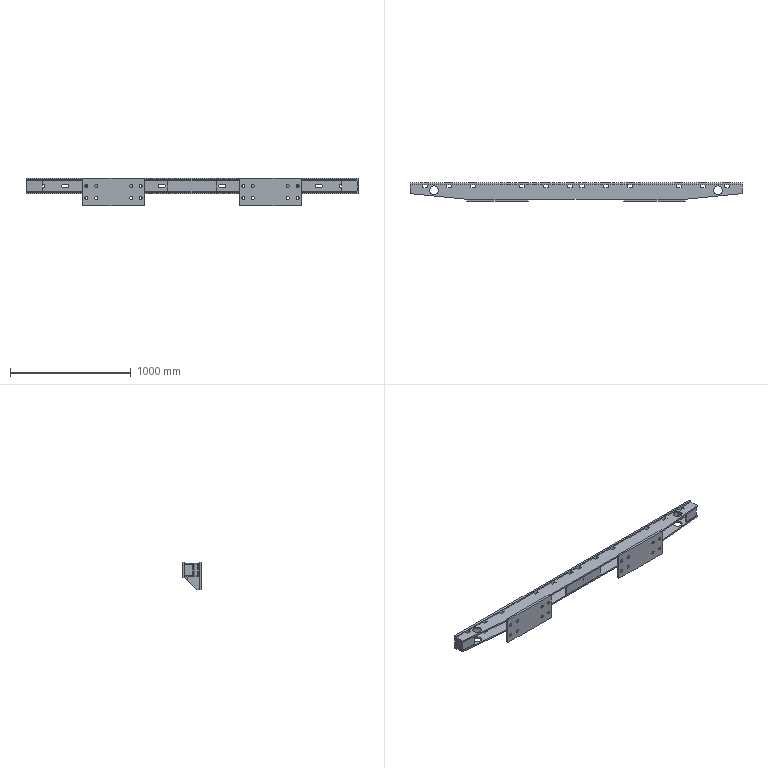Part | STEP file | Screen plate bracket (edge)_Default<As machined> | 12 solids | 280 faces | box 2750 x 152 x 230 mm | volume 16995025 mm3 | plane 216 | cylinder 64 | commonest cylinder face diameters 25 x32 24 x24 72 x8